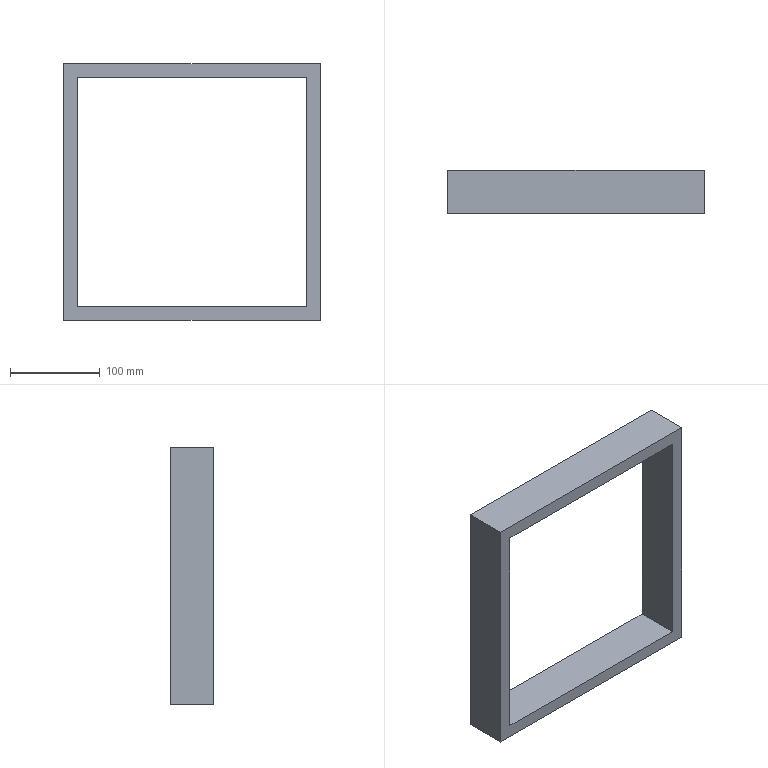Part | SolidWorks | features BaseBody 1 | 1 solid | 10 faces | box 286 x 48 x 286 mm | volume 780480 mm3 | plane 10
STEP:
#1=CARTESIAN_POINT('',(166.,44.,15.));
#2=VERTEX_POINT('',#1);
#3=CARTESIAN_POINT('',(166.,44.,271.));
#4=VERTEX_POINT('',#3);
#5=CARTESIAN_POINT('',(166.,44.,151.));
#6=DIRECTION('',(0.,0.,1.));
#7=VECTOR('',#6,1000.);
#8=LINE('',#5,#7);
#9=EDGE_CURVE('',#2,#4,#8,.T.);
#10=ORIENTED_EDGE('',*,*,#9,.T.);
#11=CARTESIAN_POINT('',(-90.,44.,271.));
#12=VERTEX_POINT('',#11);
#13=CARTESIAN_POINT('',(-92.5,44.,271.));
#14=DIRECTION('',(-1.,0.,0.));
#15=VECTOR('',#14,1000.);
#16=LINE('',#13,#15);
#17=EDGE_CURVE('',#4,#12,#16,.T.);
#18=ORIENTED_EDGE('',*,*,#17,.T.);
#19=CARTESIAN_POINT('',(-90.,44.,15.));
#20=VERTEX_POINT('',#19);
#21=CARTESIAN_POINT('',(-90.,44.,151.));
#22=DIRECTION('',(0.,0.,-1.));
#23=VECTOR('',#22,1000.);
#24=LINE('',#21,#23);
#25=EDGE_CURVE('',#12,#20,#24,.T.);
#26=ORIENTED_EDGE('',*,*,#25,.T.);
#27=CARTESIAN_POINT('',(-92.5,44.,15.));
#28=DIRECTION('',(1.,0.,0.));
#29=VECTOR('',#28,1000.);
#30=LINE('',#27,#29);
#31=EDGE_CURVE('',#20,#2,#30,.T.);
#32=ORIENTED_EDGE('',*,*,#31,.T.);
#33=EDGE_LOOP('',(#10,#18,#26,#32));
#34=FACE_BOUND('',#33,.T.);
#35=CARTESIAN_POINT('',(-105.,44.,0.));
#36=VERTEX_POINT('',#35);
#37=CARTESIAN_POINT('',(-105.,44.,286.));
#38=VERTEX_POINT('',#37);
#39=CARTESIAN_POINT('',(-105.,44.,151.));
#40=DIRECTION('',(0.,0.,1.));
#41=VECTOR('',#40,1000.);
#42=LINE('',#39,#41);
#43=EDGE_CURVE('',#36,#38,#42,.T.);
#44=ORIENTED_EDGE('',*,*,#43,.T.);
#45=CARTESIAN_POINT('',(181.,44.,286.));
#46=VERTEX_POINT('',#45);
#47=CARTESIAN_POINT('',(-92.5,44.,286.));
#48=DIRECTION('',(1.,0.,0.));
#49=VECTOR('',#48,1000.);
#50=LINE('',#47,#49);
#51=EDGE_CURVE('',#38,#46,#50,.T.);
#52=ORIENTED_EDGE('',*,*,#51,.T.);
#53=CARTESIAN_POINT('',(181.,44.,0.));
#54=VERTEX_POINT('',#53);
#55=CARTESIAN_POINT('',(181.,44.,151.));
#56=DIRECTION('',(0.,0.,-1.));
#57=VECTOR('',#56,1000.);
#58=LINE('',#55,#57);
#59=EDGE_CURVE('',#46,#54,#58,.T.);
#60=ORIENTED_EDGE('',*,*,#59,.T.);
#61=CARTESIAN_POINT('',(-92.5,44.,0.));
#62=DIRECTION('',(-1.,0.,0.));
#63=VECTOR('',#62,1000.);
#64=LINE('',#61,#63);
#65=EDGE_CURVE('',#54,#36,#64,.T.);
#66=ORIENTED_EDGE('',*,*,#65,.T.);
#67=EDGE_LOOP('',(#44,#52,#60,#66));
#68=FACE_OUTER_BOUND('',#67,.T.);
#69=CARTESIAN_POINT('',(-92.5,44.,151.));
#70=DIRECTION('',(0.,1.,0.));
#71=DIRECTION('',(0.,0.,1.));
#72=AXIS2_PLACEMENT_3D('',#69,#70,#71);
#73=PLANE('',#72);
#74=ADVANCED_FACE('',(#34,#68),#73,.T.);
#75=CARTESIAN_POINT('',(166.,-4.,271.));
#76=VERTEX_POINT('',#75);
#77=CARTESIAN_POINT('',(166.,44.,271.));
#78=DIRECTION('',(0.,-1.,0.));
#79=VECTOR('',#78,1000.);
#80=LINE('',#77,#79);
#81=EDGE_CURVE('',#4,#76,#80,.T.);
#82=ORIENTED_EDGE('',*,*,#81,.T.);
#83=CARTESIAN_POINT('',(-90.,-4.,271.));
#84=VERTEX_POINT('',#83);
#85=CARTESIAN_POINT('',(30.,-4.,271.));
#86=DIRECTION('',(-1.,0.,0.));
#87=VECTOR('',#86,1000.);
#88=LINE('',#85,#87);
#89=EDGE_CURVE('',#76,#84,#88,.T.);
#90=ORIENTED_EDGE('',*,*,#89,.T.);
#91=CARTESIAN_POINT('',(-90.,44.,271.));
#92=DIRECTION('',(0.,1.,0.));
#93=VECTOR('',#92,1000.);
#94=LINE('',#91,#93);
#95=EDGE_CURVE('',#84,#12,#94,.T.);
#96=ORIENTED_EDGE('',*,*,#95,.T.);
#97=ORIENTED_EDGE('',*,*,#17,.F.);
#98=EDGE_LOOP('',(#82,#90,#96,#97));
#99=FACE_OUTER_BOUND('',#98,.T.);
#100=CARTESIAN_POINT('',(30.,44.,271.));
#101=DIRECTION('',(0.,0.,-1.));
#102=DIRECTION('',(-1.,0.,0.));
#103=AXIS2_PLACEMENT_3D('',#100,#101,#102);
#104=PLANE('',#103);
#105=ADVANCED_FACE('',(#99),#104,.T.);
#106=CARTESIAN_POINT('',(166.,-4.,15.));
#107=VERTEX_POINT('',#106);
#108=CARTESIAN_POINT('',(166.,44.,15.));
#109=DIRECTION('',(0.,-1.,0.));
#110=VECTOR('',#109,1000.);
#111=LINE('',#108,#110);
#112=EDGE_CURVE('',#2,#107,#111,.T.);
#113=ORIENTED_EDGE('',*,*,#112,.T.);
#114=CARTESIAN_POINT('',(166.,-4.,135.));
#115=DIRECTION('',(0.,0.,1.));
#116=VECTOR('',#115,1000.);
#117=LINE('',#114,#116);
#118=EDGE_CURVE('',#107,#76,#117,.T.);
#119=ORIENTED_EDGE('',*,*,#118,.T.);
#120=ORIENTED_EDGE('',*,*,#81,.F.);
#121=ORIENTED_EDGE('',*,*,#9,.F.);
#122=EDGE_LOOP('',(#113,#119,#120,#121));
#123=FACE_OUTER_BOUND('',#122,.T.);
#124=CARTESIAN_POINT('',(166.,44.,135.));
#125=DIRECTION('',(-1.,0.,0.));
#126=DIRECTION('',(0.,0.,1.));
#127=AXIS2_PLACEMENT_3D('',#124,#125,#126);
#128=PLANE('',#127);
#129=ADVANCED_FACE('',(#123),#128,.T.);
#130=ORIENTED_EDGE('',*,*,#112,.F.);
#131=ORIENTED_EDGE('',*,*,#31,.F.);
#132=CARTESIAN_POINT('',(-90.,-4.,15.));
#133=VERTEX_POINT('',#132);
#134=CARTESIAN_POINT('',(-90.,44.,15.));
#135=DIRECTION('',(0.,-1.,0.));
#136=VECTOR('',#135,1000.);
#137=LINE('',#134,#136);
#138=EDGE_CURVE('',#20,#133,#137,.T.);
#139=ORIENTED_EDGE('',*,*,#138,.T.);
#140=CARTESIAN_POINT('',(46.,-4.,15.));
#141=DIRECTION('',(1.,0.,0.));
#142=VECTOR('',#141,1000.);
#143=LINE('',#140,#142);
#144=EDGE_CURVE('',#133,#107,#143,.T.);
#145=ORIENTED_EDGE('',*,*,#144,.T.);
#146=EDGE_LOOP('',(#130,#131,#139,#145));
#147=FACE_OUTER_BOUND('',#146,.T.);
#148=CARTESIAN_POINT('',(46.,44.,15.));
#149=DIRECTION('',(0.,0.,1.));
#150=DIRECTION('',(1.,0.,0.));
#151=AXIS2_PLACEMENT_3D('',#148,#149,#150);
#152=PLANE('',#151);
#153=ADVANCED_FACE('',(#147),#152,.T.);
#154=ORIENTED_EDGE('',*,*,#25,.F.);
#155=ORIENTED_EDGE('',*,*,#95,.F.);
#156=CARTESIAN_POINT('',(-90.,-4.,151.));
#157=DIRECTION('',(0.,0.,-1.));
#158=VECTOR('',#157,1000.);
#159=LINE('',#156,#158);
#160=EDGE_CURVE('',#84,#133,#159,.T.);
#161=ORIENTED_EDGE('',*,*,#160,.T.);
#162=ORIENTED_EDGE('',*,*,#138,.F.);
#163=EDGE_LOOP('',(#154,#155,#161,#162));
#164=FACE_OUTER_BOUND('',#163,.T.);
#165=CARTESIAN_POINT('',(-90.,44.,151.));
#166=DIRECTION('',(1.,0.,0.));
#167=DIRECTION('',(0.,0.,-1.));
#168=AXIS2_PLACEMENT_3D('',#165,#166,#167);
#169=PLANE('',#168);
#170=ADVANCED_FACE('',(#164),#169,.T.);
#171=CARTESIAN_POINT('',(-105.,-4.,286.));
#172=VERTEX_POINT('',#171);
#173=CARTESIAN_POINT('',(-105.,20.,286.));
#174=DIRECTION('',(0.,-1.,0.));
#175=VECTOR('',#174,1000.);
#176=LINE('',#173,#175);
#177=EDGE_CURVE('',#38,#172,#176,.T.);
#178=ORIENTED_EDGE('',*,*,#177,.T.);
#179=CARTESIAN_POINT('',(181.,-4.,286.));
#180=VERTEX_POINT('',#179);
#181=CARTESIAN_POINT('',(-92.5,-4.,286.));
#182=DIRECTION('',(1.,0.,0.));
#183=VECTOR('',#182,1000.);
#184=LINE('',#181,#183);
#185=EDGE_CURVE('',#172,#180,#184,.T.);
#186=ORIENTED_EDGE('',*,*,#185,.T.);
#187=CARTESIAN_POINT('',(181.,20.,286.));
#188=DIRECTION('',(0.,1.,0.));
#189=VECTOR('',#188,1000.);
#190=LINE('',#187,#189);
#191=EDGE_CURVE('',#180,#46,#190,.T.);
#192=ORIENTED_EDGE('',*,*,#191,.T.);
#193=ORIENTED_EDGE('',*,*,#51,.F.);
#194=EDGE_LOOP('',(#178,#186,#192,#193));
#195=FACE_OUTER_BOUND('',#194,.T.);
#196=CARTESIAN_POINT('',(-92.5,20.,286.));
#197=DIRECTION('',(0.,0.,1.));
#198=DIRECTION('',(1.,0.,0.));
#199=AXIS2_PLACEMENT_3D('',#196,#197,#198);
#200=PLANE('',#199);
#201=ADVANCED_FACE('',(#195),#200,.T.);
#202=ORIENTED_EDGE('',*,*,#43,.F.);
#203=CARTESIAN_POINT('',(-105.,-4.,0.));
#204=VERTEX_POINT('',#203);
#205=CARTESIAN_POINT('',(-105.,20.,0.));
#206=DIRECTION('',(0.,-1.,0.));
#207=VECTOR('',#206,1000.);
#208=LINE('',#205,#207);
#209=EDGE_CURVE('',#36,#204,#208,.T.);
#210=ORIENTED_EDGE('',*,*,#209,.T.);
#211=CARTESIAN_POINT('',(-105.,-4.,151.));
#212=DIRECTION('',(0.,0.,1.));
#213=VECTOR('',#212,1000.);
#214=LINE('',#211,#213);
#215=EDGE_CURVE('',#204,#172,#214,.T.);
#216=ORIENTED_EDGE('',*,*,#215,.T.);
#217=ORIENTED_EDGE('',*,*,#177,.F.);
#218=EDGE_LOOP('',(#202,#210,#216,#217));
#219=FACE_OUTER_BOUND('',#218,.T.);
#220=CARTESIAN_POINT('',(-105.,20.,151.));
#221=DIRECTION('',(-1.,0.,0.));
#222=DIRECTION('',(0.,0.,1.));
#223=AXIS2_PLACEMENT_3D('',#220,#221,#222);
#224=PLANE('',#223);
#225=ADVANCED_FACE('',(#219),#224,.T.);
#226=ORIENTED_EDGE('',*,*,#209,.F.);
#227=ORIENTED_EDGE('',*,*,#65,.F.);
#228=CARTESIAN_POINT('',(181.,-4.,0.));
#229=VERTEX_POINT('',#228);
#230=CARTESIAN_POINT('',(181.,44.,0.));
#231=DIRECTION('',(0.,-1.,0.));
#232=VECTOR('',#231,1000.);
#233=LINE('',#230,#232);
#234=EDGE_CURVE('',#54,#229,#233,.T.);
#235=ORIENTED_EDGE('',*,*,#234,.T.);
#236=CARTESIAN_POINT('',(670.,-4.,0.));
#237=DIRECTION('',(-1.,0.,0.));
#238=VECTOR('',#237,1000.);
#239=LINE('',#236,#238);
#240=EDGE_CURVE('',#229,#204,#239,.T.);
#241=ORIENTED_EDGE('',*,*,#240,.T.);
#242=EDGE_LOOP('',(#226,#227,#235,#241));
#243=FACE_OUTER_BOUND('',#242,.T.);
#244=CARTESIAN_POINT('',(670.,44.,0.));
#245=DIRECTION('',(0.,0.,-1.));
#246=DIRECTION('',(-1.,0.,0.));
#247=AXIS2_PLACEMENT_3D('',#244,#245,#246);
#248=PLANE('',#247);
#249=ADVANCED_FACE('',(#243),#248,.T.);
#250=ORIENTED_EDGE('',*,*,#191,.F.);
#251=CARTESIAN_POINT('',(181.,-4.,12.5));
#252=DIRECTION('',(0.,0.,-1.));
#253=VECTOR('',#252,1000.);
#254=LINE('',#251,#253);
#255=EDGE_CURVE('',#180,#229,#254,.T.);
#256=ORIENTED_EDGE('',*,*,#255,.T.);
#257=ORIENTED_EDGE('',*,*,#234,.F.);
#258=ORIENTED_EDGE('',*,*,#59,.F.);
#259=EDGE_LOOP('',(#250,#256,#257,#258));
#260=FACE_OUTER_BOUND('',#259,.T.);
#261=CARTESIAN_POINT('',(181.,20.,12.5));
#262=DIRECTION('',(1.,0.,0.));
#263=DIRECTION('',(0.,0.,-1.));
#264=AXIS2_PLACEMENT_3D('',#261,#262,#263);
#265=PLANE('',#264);
#266=ADVANCED_FACE('',(#260),#265,.T.);
#267=ORIENTED_EDGE('',*,*,#118,.F.);
#268=ORIENTED_EDGE('',*,*,#144,.F.);
#269=ORIENTED_EDGE('',*,*,#160,.F.);
#270=ORIENTED_EDGE('',*,*,#89,.F.);
#271=EDGE_LOOP('',(#267,#268,#269,#270));
#272=FACE_BOUND('',#271,.T.);
#273=ORIENTED_EDGE('',*,*,#215,.F.);
#274=ORIENTED_EDGE('',*,*,#240,.F.);
#275=ORIENTED_EDGE('',*,*,#255,.F.);
#276=ORIENTED_EDGE('',*,*,#185,.F.);
#277=EDGE_LOOP('',(#273,#274,#275,#276));
#278=FACE_OUTER_BOUND('',#277,.T.);
#279=CARTESIAN_POINT('',(-92.5,-4.,151.));
#280=DIRECTION('',(0.,-1.,0.));
#281=DIRECTION('',(0.,0.,-1.));
#282=AXIS2_PLACEMENT_3D('',#279,#280,#281);
#283=PLANE('',#282);
#284=ADVANCED_FACE('',(#272,#278),#283,.T.);
#285=CLOSED_SHELL('',(#74,#105,#129,#153,#170,#201,#225,#249,#266,#284));
#286=MANIFOLD_SOLID_BREP('',#285);
#287=CARTESIAN_POINT('',(0.,0.,0.));
#288=DIRECTION('',(0.,0.,1.));
#289=DIRECTION('',(1.,0.,0.));
#290=AXIS2_PLACEMENT_3D('',#287,#288,#289);
#291=(LENGTH_UNIT()NAMED_UNIT(*)SI_UNIT(.MILLI.,.METRE.));
#292=UNCERTAINTY_MEASURE_WITH_UNIT(LENGTH_MEASURE(0.00001),#291,'','');
#293=(NAMED_UNIT(*)PLANE_ANGLE_UNIT()SI_UNIT($,.RADIAN.));
#294=(NAMED_UNIT(*)SI_UNIT($,.STERADIAN.)SOLID_ANGLE_UNIT());
#295=(GEOMETRIC_REPRESENTATION_CONTEXT(3)GLOBAL_UNCERTAINTY_ASSIGNED_CONTEXT((#292))GLOBAL_UNIT_ASSIGNED_CONTEXT((#291,#293,#294))REPRESENTATION_CONTEXT('',''));
#296=ADVANCED_BREP_SHAPE_REPRESENTATION('',(#286,#290),#295);